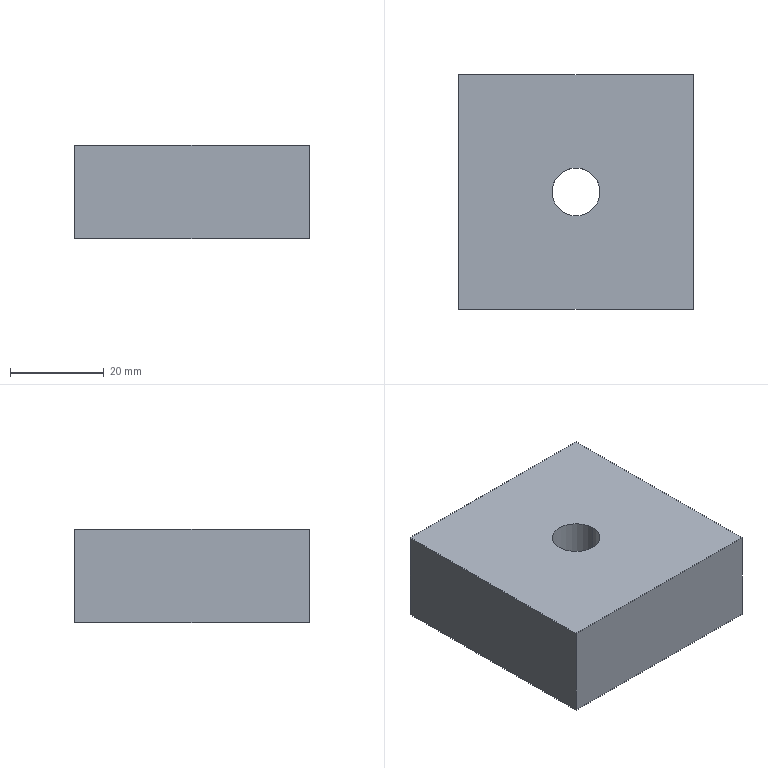Part | SolidWorks | features FlatPattern 1, HoleWzd 1, SMBaseFlange 1, SheetMetal 1 | 1 solid | 8 faces | box 50 x 50 x 20 mm | volume 48366 mm3 | plane 6 | cylinder 2 | commonest cylinder face diameters 10.2 x2
STEP:
#1=CARTESIAN_POINT('',(-5.1,0.,-20.));
#2=VERTEX_POINT('',#1);
#3=CARTESIAN_POINT('',(5.1,0.,-20.));
#4=VERTEX_POINT('',#3);
#5=CARTESIAN_POINT('',(0.,0.,-20.));
#6=DIRECTION('',(0.,0.,1.));
#7=DIRECTION('',(1.,0.,0.));
#8=AXIS2_PLACEMENT_3D('',#5,#6,#7);
#9=CIRCLE('',#8,5.1);
#10=EDGE_CURVE('',#2,#4,#9,.T.);
#11=ORIENTED_EDGE('',*,*,#10,.F.);
#12=CARTESIAN_POINT('',(-5.1,0.,0.));
#13=VERTEX_POINT('',#12);
#14=CARTESIAN_POINT('',(-5.1,0.,0.));
#15=DIRECTION('',(0.,0.,1.));
#16=VECTOR('',#15,1000.);
#17=LINE('',#14,#16);
#18=EDGE_CURVE('',#2,#13,#17,.T.);
#19=ORIENTED_EDGE('',*,*,#18,.T.);
#20=CARTESIAN_POINT('',(5.1,0.,0.));
#21=VERTEX_POINT('',#20);
#22=CARTESIAN_POINT('',(0.,0.,0.));
#23=DIRECTION('',(0.,0.,1.));
#24=DIRECTION('',(1.,0.,0.));
#25=AXIS2_PLACEMENT_3D('',#22,#23,#24);
#26=CIRCLE('',#25,5.1);
#27=EDGE_CURVE('',#13,#21,#26,.T.);
#28=ORIENTED_EDGE('',*,*,#27,.T.);
#29=CARTESIAN_POINT('',(5.1,0.,0.));
#30=DIRECTION('',(0.,0.,1.));
#31=VECTOR('',#30,1000.);
#32=LINE('',#29,#31);
#33=EDGE_CURVE('',#4,#21,#32,.T.);
#34=ORIENTED_EDGE('',*,*,#33,.F.);
#35=EDGE_LOOP('',(#11,#19,#28,#34));
#36=FACE_OUTER_BOUND('',#35,.T.);
#37=CARTESIAN_POINT('',(0.,0.,0.));
#38=DIRECTION('',(0.,0.,1.));
#39=DIRECTION('',(1.,0.,0.));
#40=AXIS2_PLACEMENT_3D('',#37,#38,#39);
#41=CYLINDRICAL_SURFACE('',#40,5.1);
#42=ADVANCED_FACE('',(#36),#41,.F.);
#43=CARTESIAN_POINT('',(25.,-25.,0.));
#44=VERTEX_POINT('',#43);
#45=CARTESIAN_POINT('',(25.,25.,0.));
#46=VERTEX_POINT('',#45);
#47=CARTESIAN_POINT('',(25.,25.,0.));
#48=DIRECTION('',(0.,1.,0.));
#49=VECTOR('',#48,1000.);
#50=LINE('',#47,#49);
#51=EDGE_CURVE('',#44,#46,#50,.T.);
#52=ORIENTED_EDGE('',*,*,#51,.F.);
#53=CARTESIAN_POINT('',(25.,-25.,-20.));
#54=VERTEX_POINT('',#53);
#55=CARTESIAN_POINT('',(25.,-25.,-20.));
#56=DIRECTION('',(0.,0.,1.));
#57=VECTOR('',#56,1000.);
#58=LINE('',#55,#57);
#59=EDGE_CURVE('',#54,#44,#58,.T.);
#60=ORIENTED_EDGE('',*,*,#59,.F.);
#61=CARTESIAN_POINT('',(25.,25.,-20.));
#62=VERTEX_POINT('',#61);
#63=CARTESIAN_POINT('',(25.,25.,-20.));
#64=DIRECTION('',(0.,1.,0.));
#65=VECTOR('',#64,1000.);
#66=LINE('',#63,#65);
#67=EDGE_CURVE('',#54,#62,#66,.T.);
#68=ORIENTED_EDGE('',*,*,#67,.T.);
#69=CARTESIAN_POINT('',(25.,25.,-20.));
#70=DIRECTION('',(0.,0.,1.));
#71=VECTOR('',#70,1000.);
#72=LINE('',#69,#71);
#73=EDGE_CURVE('',#62,#46,#72,.T.);
#74=ORIENTED_EDGE('',*,*,#73,.T.);
#75=EDGE_LOOP('',(#52,#60,#68,#74));
#76=FACE_OUTER_BOUND('',#75,.T.);
#77=CARTESIAN_POINT('',(25.,25.,-20.));
#78=DIRECTION('',(1.,0.,0.));
#79=DIRECTION('',(0.,1.,0.));
#80=AXIS2_PLACEMENT_3D('',#77,#78,#79);
#81=PLANE('',#80);
#82=ADVANCED_FACE('',(#76),#81,.T.);
#83=CARTESIAN_POINT('',(-25.,-25.,0.));
#84=VERTEX_POINT('',#83);
#85=CARTESIAN_POINT('',(-25.,-25.,0.));
#86=DIRECTION('',(1.,0.,0.));
#87=VECTOR('',#86,1000.);
#88=LINE('',#85,#87);
#89=EDGE_CURVE('',#84,#44,#88,.T.);
#90=ORIENTED_EDGE('',*,*,#89,.F.);
#91=CARTESIAN_POINT('',(-25.,-25.,-20.));
#92=VERTEX_POINT('',#91);
#93=CARTESIAN_POINT('',(-25.,-25.,-20.));
#94=DIRECTION('',(0.,0.,1.));
#95=VECTOR('',#94,1000.);
#96=LINE('',#93,#95);
#97=EDGE_CURVE('',#92,#84,#96,.T.);
#98=ORIENTED_EDGE('',*,*,#97,.F.);
#99=CARTESIAN_POINT('',(-25.,-25.,-20.));
#100=DIRECTION('',(1.,0.,0.));
#101=VECTOR('',#100,1000.);
#102=LINE('',#99,#101);
#103=EDGE_CURVE('',#92,#54,#102,.T.);
#104=ORIENTED_EDGE('',*,*,#103,.T.);
#105=ORIENTED_EDGE('',*,*,#59,.T.);
#106=EDGE_LOOP('',(#90,#98,#104,#105));
#107=FACE_OUTER_BOUND('',#106,.T.);
#108=CARTESIAN_POINT('',(-25.,-25.,-20.));
#109=DIRECTION('',(0.,-1.,0.));
#110=DIRECTION('',(0.,0.,-1.));
#111=AXIS2_PLACEMENT_3D('',#108,#109,#110);
#112=PLANE('',#111);
#113=ADVANCED_FACE('',(#107),#112,.T.);
#114=CARTESIAN_POINT('',(-25.,25.,0.));
#115=VERTEX_POINT('',#114);
#116=CARTESIAN_POINT('',(-25.,25.,0.));
#117=DIRECTION('',(0.,-1.,0.));
#118=VECTOR('',#117,1000.);
#119=LINE('',#116,#118);
#120=EDGE_CURVE('',#115,#84,#119,.T.);
#121=ORIENTED_EDGE('',*,*,#120,.F.);
#122=CARTESIAN_POINT('',(-25.,25.,-20.));
#123=VERTEX_POINT('',#122);
#124=CARTESIAN_POINT('',(-25.,25.,-20.));
#125=DIRECTION('',(0.,0.,1.));
#126=VECTOR('',#125,1000.);
#127=LINE('',#124,#126);
#128=EDGE_CURVE('',#123,#115,#127,.T.);
#129=ORIENTED_EDGE('',*,*,#128,.F.);
#130=CARTESIAN_POINT('',(-25.,25.,-20.));
#131=DIRECTION('',(0.,-1.,0.));
#132=VECTOR('',#131,1000.);
#133=LINE('',#130,#132);
#134=EDGE_CURVE('',#123,#92,#133,.T.);
#135=ORIENTED_EDGE('',*,*,#134,.T.);
#136=ORIENTED_EDGE('',*,*,#97,.T.);
#137=EDGE_LOOP('',(#121,#129,#135,#136));
#138=FACE_OUTER_BOUND('',#137,.T.);
#139=CARTESIAN_POINT('',(-25.,25.,-20.));
#140=DIRECTION('',(-1.,0.,0.));
#141=DIRECTION('',(0.,-1.,0.));
#142=AXIS2_PLACEMENT_3D('',#139,#140,#141);
#143=PLANE('',#142);
#144=ADVANCED_FACE('',(#138),#143,.T.);
#145=CARTESIAN_POINT('',(-25.,25.,0.));
#146=DIRECTION('',(-1.,0.,0.));
#147=VECTOR('',#146,1000.);
#148=LINE('',#145,#147);
#149=EDGE_CURVE('',#46,#115,#148,.T.);
#150=ORIENTED_EDGE('',*,*,#149,.F.);
#151=ORIENTED_EDGE('',*,*,#73,.F.);
#152=CARTESIAN_POINT('',(-25.,25.,-20.));
#153=DIRECTION('',(-1.,0.,0.));
#154=VECTOR('',#153,1000.);
#155=LINE('',#152,#154);
#156=EDGE_CURVE('',#62,#123,#155,.T.);
#157=ORIENTED_EDGE('',*,*,#156,.T.);
#158=ORIENTED_EDGE('',*,*,#128,.T.);
#159=EDGE_LOOP('',(#150,#151,#157,#158));
#160=FACE_OUTER_BOUND('',#159,.T.);
#161=CARTESIAN_POINT('',(-25.,25.,-20.));
#162=DIRECTION('',(0.,1.,0.));
#163=DIRECTION('',(0.,0.,1.));
#164=AXIS2_PLACEMENT_3D('',#161,#162,#163);
#165=PLANE('',#164);
#166=ADVANCED_FACE('',(#160),#165,.T.);
#167=CARTESIAN_POINT('',(0.,0.,-20.));
#168=DIRECTION('',(0.,0.,1.));
#169=DIRECTION('',(1.,0.,0.));
#170=AXIS2_PLACEMENT_3D('',#167,#168,#169);
#171=CIRCLE('',#170,5.1);
#172=EDGE_CURVE('',#4,#2,#171,.T.);
#173=ORIENTED_EDGE('',*,*,#172,.T.);
#174=ORIENTED_EDGE('',*,*,#10,.T.);
#175=EDGE_LOOP('',(#173,#174));
#176=FACE_BOUND('',#175,.T.);
#177=ORIENTED_EDGE('',*,*,#67,.F.);
#178=ORIENTED_EDGE('',*,*,#103,.F.);
#179=ORIENTED_EDGE('',*,*,#134,.F.);
#180=ORIENTED_EDGE('',*,*,#156,.F.);
#181=EDGE_LOOP('',(#177,#178,#179,#180));
#182=FACE_OUTER_BOUND('',#181,.T.);
#183=CARTESIAN_POINT('',(0.,0.,-20.));
#184=DIRECTION('',(0.,0.,1.));
#185=DIRECTION('',(1.,0.,0.));
#186=AXIS2_PLACEMENT_3D('',#183,#184,#185);
#187=PLANE('',#186);
#188=ADVANCED_FACE('',(#176,#182),#187,.F.);
#189=CARTESIAN_POINT('',(0.,0.,0.));
#190=DIRECTION('',(0.,0.,1.));
#191=DIRECTION('',(1.,0.,0.));
#192=AXIS2_PLACEMENT_3D('',#189,#190,#191);
#193=CIRCLE('',#192,5.1);
#194=EDGE_CURVE('',#21,#13,#193,.T.);
#195=ORIENTED_EDGE('',*,*,#194,.F.);
#196=ORIENTED_EDGE('',*,*,#27,.F.);
#197=EDGE_LOOP('',(#195,#196));
#198=FACE_BOUND('',#197,.T.);
#199=ORIENTED_EDGE('',*,*,#51,.T.);
#200=ORIENTED_EDGE('',*,*,#149,.T.);
#201=ORIENTED_EDGE('',*,*,#120,.T.);
#202=ORIENTED_EDGE('',*,*,#89,.T.);
#203=EDGE_LOOP('',(#199,#200,#201,#202));
#204=FACE_OUTER_BOUND('',#203,.T.);
#205=CARTESIAN_POINT('',(0.,0.,0.));
#206=DIRECTION('',(0.,0.,1.));
#207=DIRECTION('',(1.,0.,0.));
#208=AXIS2_PLACEMENT_3D('',#205,#206,#207);
#209=PLANE('',#208);
#210=ADVANCED_FACE('',(#198,#204),#209,.T.);
#211=ORIENTED_EDGE('',*,*,#18,.F.);
#212=ORIENTED_EDGE('',*,*,#172,.F.);
#213=ORIENTED_EDGE('',*,*,#33,.T.);
#214=ORIENTED_EDGE('',*,*,#194,.T.);
#215=EDGE_LOOP('',(#211,#212,#213,#214));
#216=FACE_OUTER_BOUND('',#215,.T.);
#217=CARTESIAN_POINT('',(0.,0.,0.));
#218=DIRECTION('',(0.,0.,1.));
#219=DIRECTION('',(1.,0.,0.));
#220=AXIS2_PLACEMENT_3D('',#217,#218,#219);
#221=CYLINDRICAL_SURFACE('',#220,5.1);
#222=ADVANCED_FACE('',(#216),#221,.F.);
#223=CLOSED_SHELL('',(#42,#82,#113,#144,#166,#188,#210,#222));
#224=MANIFOLD_SOLID_BREP('',#223);
#225=CARTESIAN_POINT('',(0.,0.,0.));
#226=DIRECTION('',(0.,0.,1.));
#227=DIRECTION('',(1.,0.,0.));
#228=AXIS2_PLACEMENT_3D('',#225,#226,#227);
#229=(LENGTH_UNIT()NAMED_UNIT(*)SI_UNIT(.MILLI.,.METRE.));
#230=UNCERTAINTY_MEASURE_WITH_UNIT(LENGTH_MEASURE(0.00001),#229,'','');
#231=(NAMED_UNIT(*)PLANE_ANGLE_UNIT()SI_UNIT($,.RADIAN.));
#232=(NAMED_UNIT(*)SI_UNIT($,.STERADIAN.)SOLID_ANGLE_UNIT());
#233=(GEOMETRIC_REPRESENTATION_CONTEXT(3)GLOBAL_UNCERTAINTY_ASSIGNED_CONTEXT((#230))GLOBAL_UNIT_ASSIGNED_CONTEXT((#229,#231,#232))REPRESENTATION_CONTEXT('',''));
#234=ADVANCED_BREP_SHAPE_REPRESENTATION('',(#224,#228),#233);